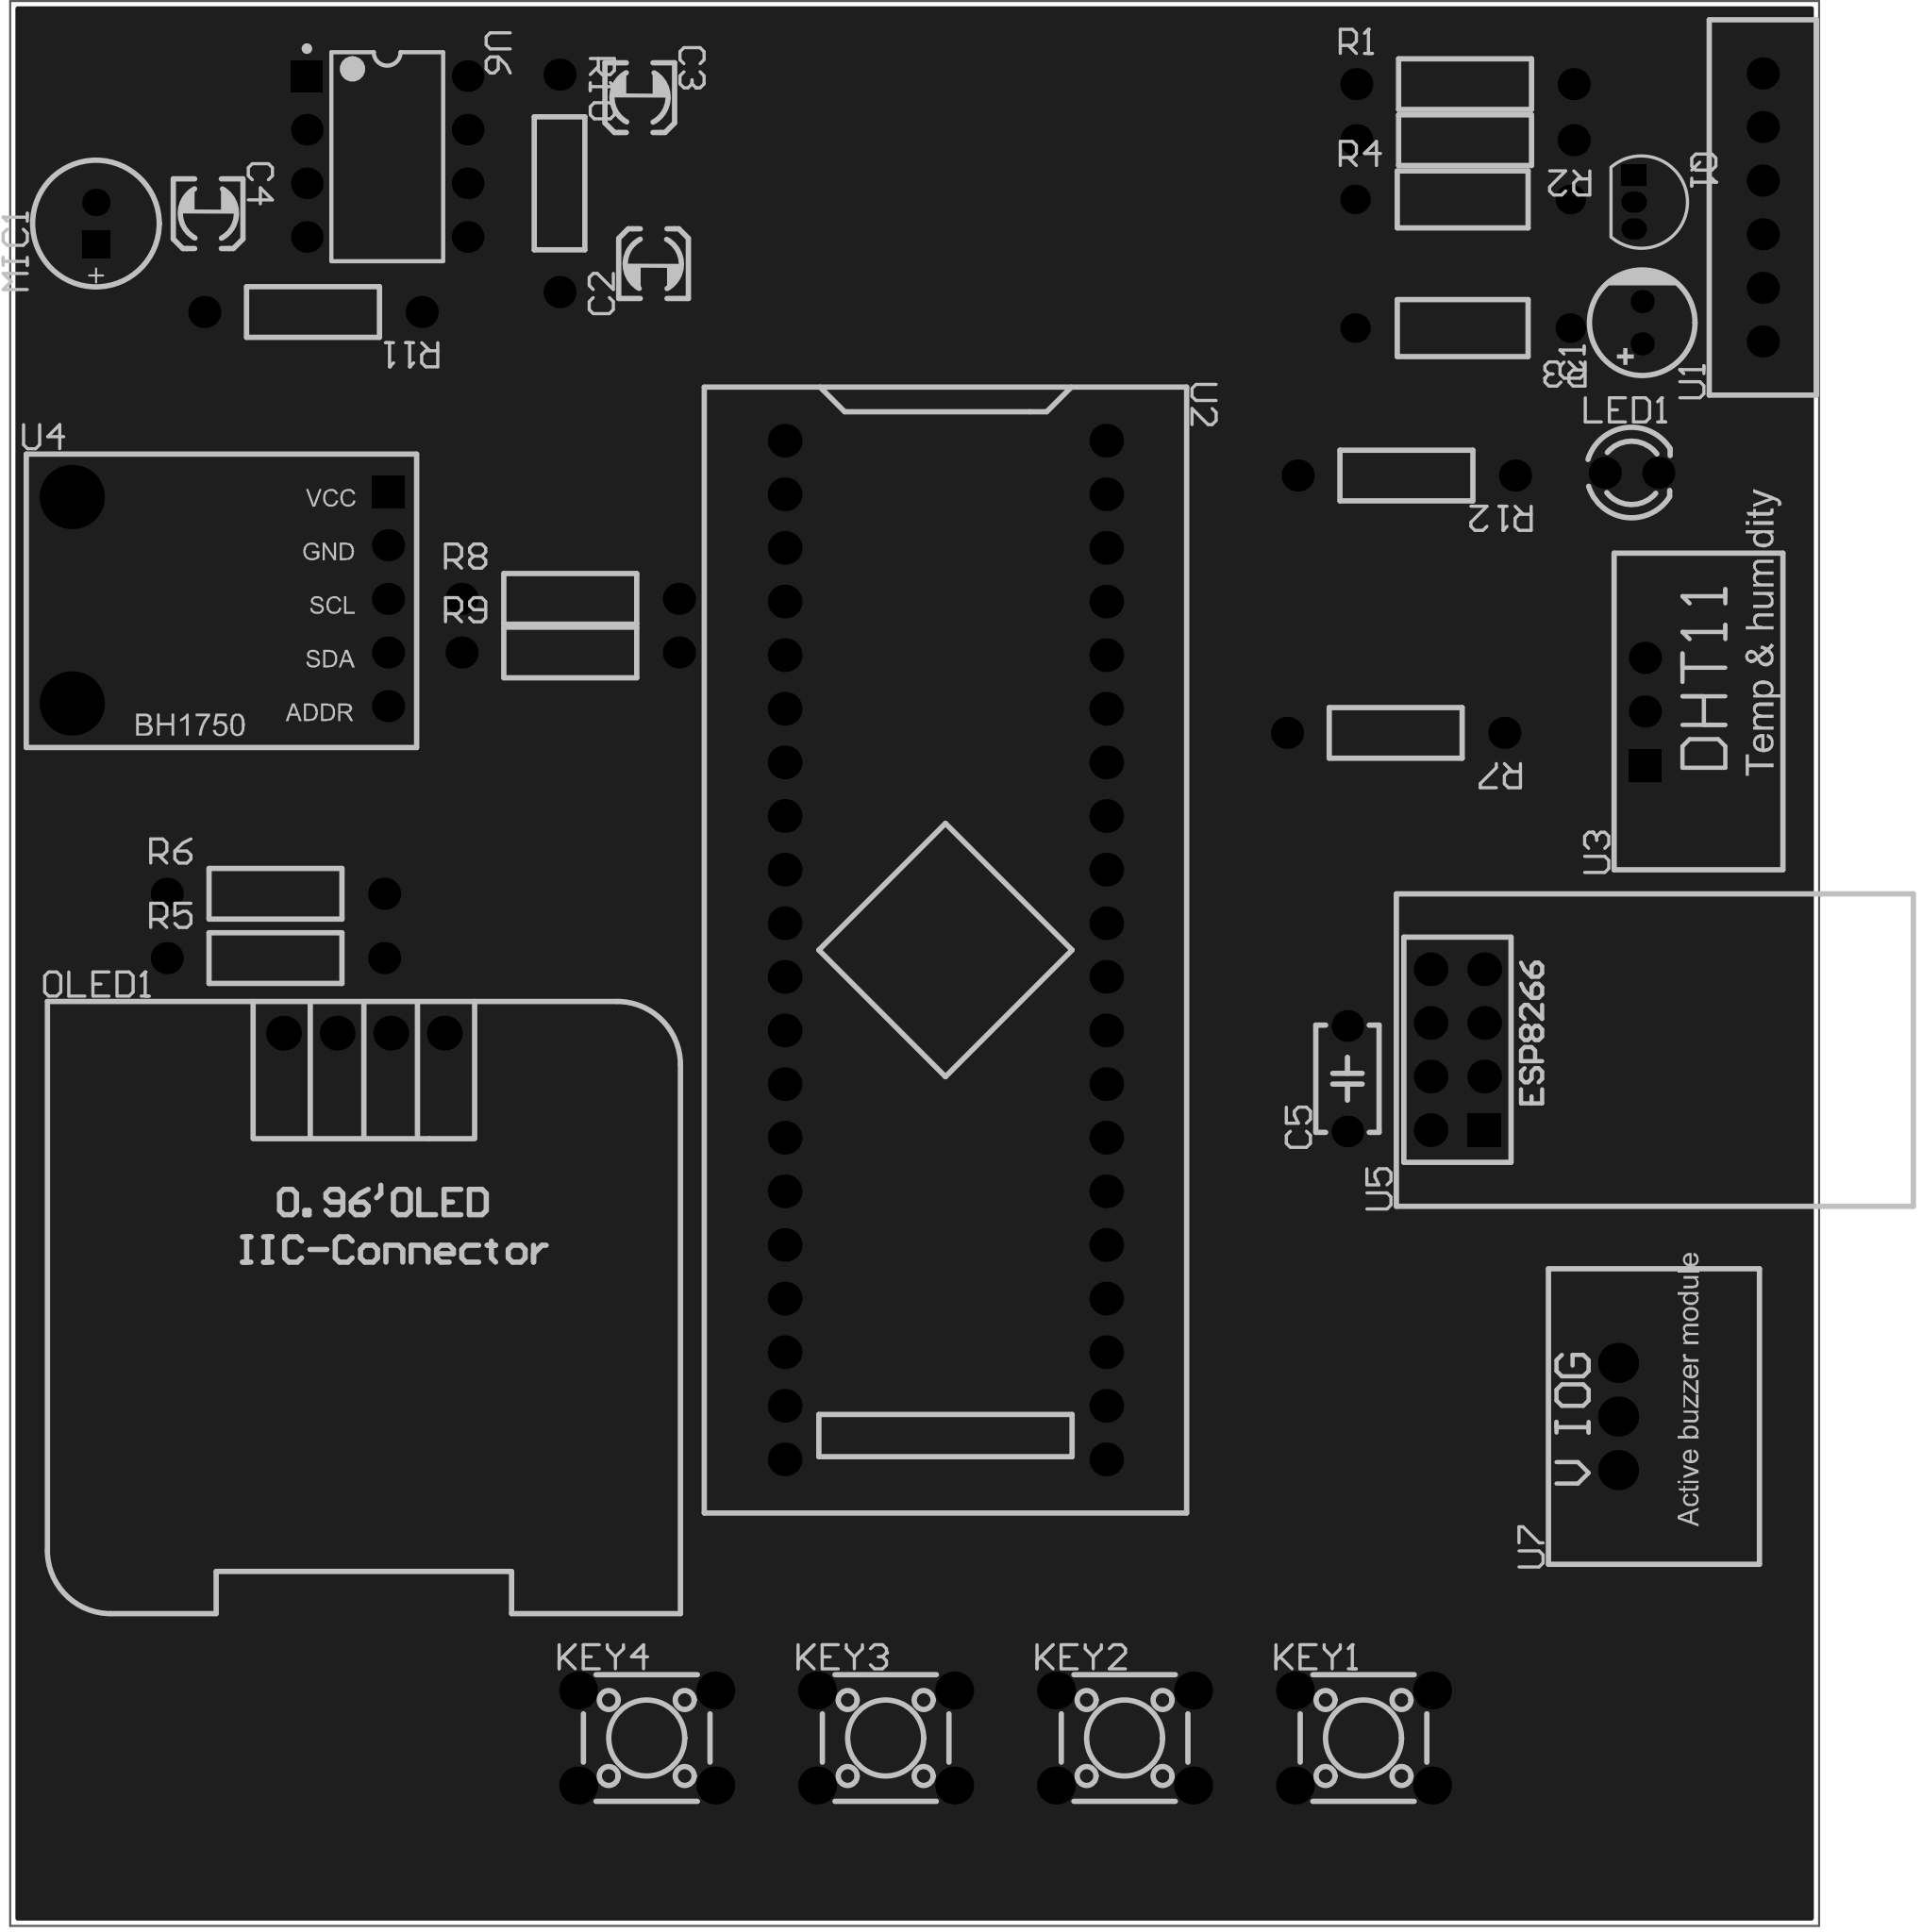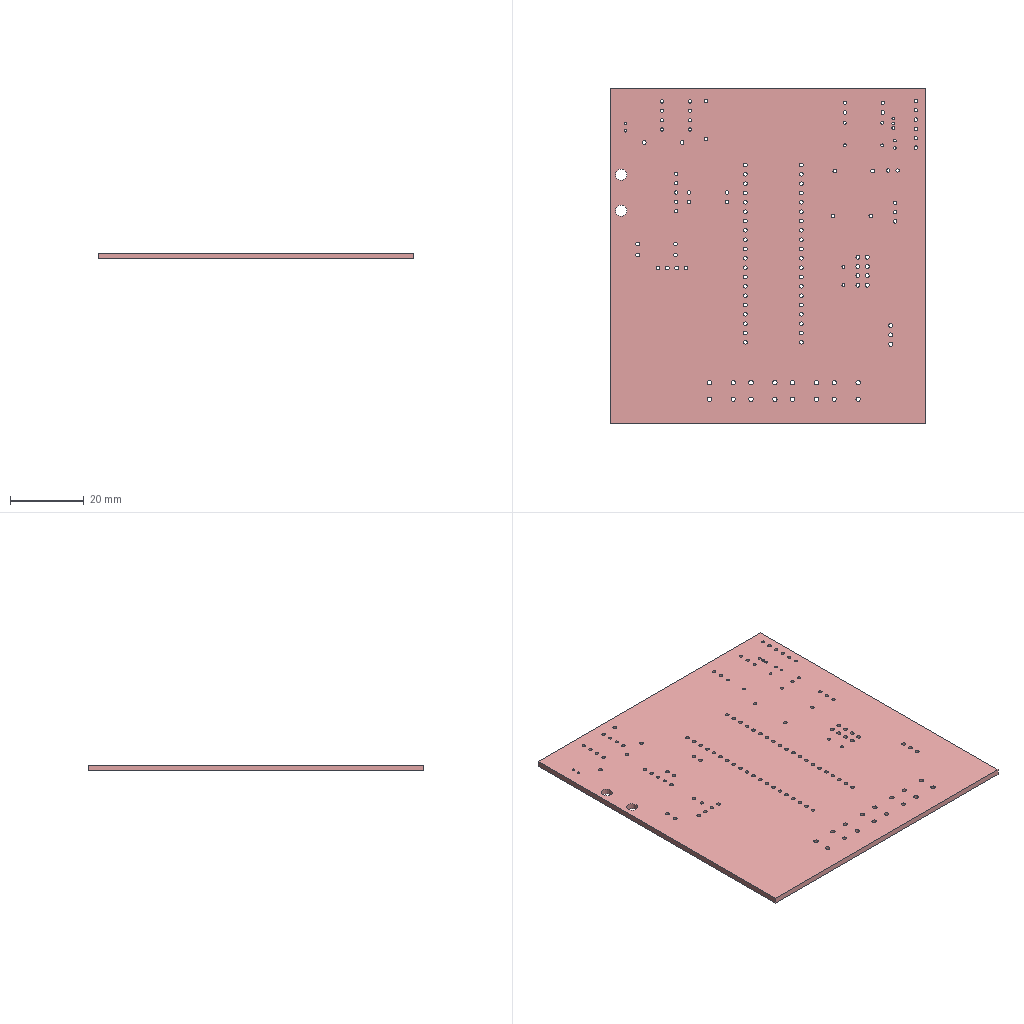Circuit board layout | Altium Designer | box 85.7 x 91.2 x 1.6 mm
Layer stack:
# Altium Designer layer stack of  (unit mm; dielectric type: 0 none, 1 core, 2 prepreg, 3 surface material)
index,name,kind,layer,copper_thickness_mm,dielectric_type,dielectric_thickness_mm,dielectric_material,dielectric_constant
0,Top Paste Mask Layer,other,,,,,,
1,Top Silkscreen Layer,other,,,,,,
2,Top Solder Mask Layer,dielectric,,,3,0.01,,3.3
3,Top Layer,copper,Top Layer,0.035,,,,
4,Dielectric1,dielectric,,,3,1.51,FR4,4.5
5,Bottom Layer,copper,Bottom Layer,0.035,,,,
6,Bottom Solder Mask Layer,dielectric,,,3,0.01,,3.3
7,Bottom Silkscreen Layer,other,,,,,,
8,Bottom Paste Mask Layer,other,,,,,,
# drill layer pairs: low layer,high layer
drill_pair,Top Layer,Bottom Layer
Part placement:
Designator,Comment,Layer,Footprint,Center-X(mm),Center-Y(mm),Rotation
C1,10uF,TopLayer,CAP-TH_BD5.0-P2.00-D0.5-FD,158.877,160.782,90
C2,10uF,TopLayer,C_Ele_SMD_3x5.4mm,112.028,163.581,90
C3,10uF,TopLayer,C_Ele_SMD_3x5.4mm,111.365,171.445,270
C4,10uF,TopLayer,C_Ele_SMD_3x5.4mm,90.909,165.947,270
C5,5pF,TopLayer,CAP-TH_L5.0-W3.0-P5.00-D0.6,144.907,124.968,90
KEY1,,TopLayer,SW-TH_4P-L6.0-W6.0-P4.50-LS6.5,145.669,93.736,0
KEY2,,TopLayer,SW-TH_4P-L6.0-W6.0-P4.50-LS6.5,134.346,93.736,0
KEY3,,TopLayer,SW-TH_4P-L6.0-W6.0-P4.50-LS6.5,123.023,93.736,0
KEY4,,TopLayer,SW-TH_4P-L6.0-W6.0-P4.50-LS6.5,111.7,93.736,0
LED1,,TopLayer,LED_TH-3mm,158.369,153.67,0
MIC1,MIC,TopLayer,MIC-TH_BD6.0-P2.00,85.598,165.481,90
OLED1,0.96OLED_4P_MODULE_JX,TopLayer,0.96OLED_4P,98.298,127.127,0
Q1,S8050,TopLayer,TO-92-3_L4.5-W3.5-P1.27-L,158.496,166.497,270
R1,10kΩ,TopLayer,Res_1/4W,150.48,172.085,0
R2,10kΩ,TopLayer,Res_1/4W,150.48,169.429,180
R3,10kΩ,TopLayer,RES-TH_BD2.7-L6.2-P10.20-D0.4,150.368,160.528,180
R4,1kΩ,TopLayer,RES-TH_BD2.7-L6.2-P10.20-D0.4,150.368,166.624,0
R5,10kΩ,TopLayer,Res_1/4W,94.107,130.683,0
R6,10kΩ,TopLayer,Res_1/4W,94.107,133.731,0
R7,4.7K,TopLayer,Res_1/4W,147.193,141.351,180
R8,10kΩ,TopLayer,Res_1/4W,108.077,147.701,0
R9,10kΩ,TopLayer,Res_1/4W,108.077,145.161,0
R10,3kΩ,TopLayer,Res_1/4W,107.569,167.386,270
R11,100kΩ,TopLayer,Res_1/4W,95.885,161.29,180
R12,10kΩ,TopLayer,Res_1/4W,147.701,153.543,180
U1,PM2.5 sensor_GP2Y1014AU,TopLayer,PM2.5传感器_GP2Y1014AU,164.592,166.243,90
U2,STM32F103C8T6-Card,TopLayer,CONN-TH_L53.3-W22.9_STM32F103C8T6-CARD,125.857,131.064,270
U3,DHT11,TopLayer,DHT11,159.004,142.367,90
U4,,TopLayer,BH1750光照传感器,91.948,147.701,0
U5,,TopLayer,ESP8266-1,150.119,126.342,90
U6,LM386N-3/NOPB,TopLayer,DIP-8_L9.8-W6.6-P2.54-LS7.6-BL,99.404,168.656,270
U7,,TopLayer,有源蜂鸣器模块,157.734,108.966,90
Pad and via stacks:
# Altium Designer via and pad stacks of  (unit mm). Each distinct definition once, with the count of objects using it.
# via: kind,start_layer,end_layer,hole_mm,diameter_mm,mode(0 simple;1 top-mid-bottom;2 full stack),diameter_per_layer,count,example_net
# pad: kind,layer,hole_mm,hole_type(0 round;1 square;2 slot),plating,top_size,top_shape(1 round;2 rect;3 octagon;9 rounded rect),mid_size,bottom_size,mode,footprint,size_per_layer,count,example
pad,Multi-Layer,0.7,0,plated,1.1x1.1,1,1.1x1.1,1.1x1.1,0,CAP-TH_BD5.0-P2.00-D0.5-FD,,2,C1.1
pad,Multi-Layer,0.8,0,plated,1.5x1.5,1,1.5x1.5,1.5x1.5,0,CAP-TH_L5.0-W3.0-P5.00-D0.6,,2,C5.2
pad,Multi-Layer,1.2,0,plated,1.8x1.8,1,1.8x1.8,1.8x1.8,0,SW-TH_4P-L6.0-W6.0-P4.50-LS6.5,,16,KEY1.1
pad,Multi-Layer,0.9144,0,plated,1.524x1.524,1,1.524x1.524,1.524x1.524,0,LED_TH-3mm,,2,LED1.1
pad,Multi-Layer,0.7,0,plated,1.3x1.3,2,1.3x1.3,1.3x1.3,0,MIC-TH_BD6.0-P2.00,,1,MIC1.1
pad,Multi-Layer,0.7,0,plated,1.3x1.3,1,1.3x1.3,1.3x1.3,0,MIC-TH_BD6.0-P2.00,,1,MIC1.2
pad,Multi-Layer,1,0,plated,1.65x1.65,1,1.65x1.65,1.65x1.65,0,0.96OLED_4P,,4,OLED1.4
pad,Multi-Layer,0.7,2,plated,1x1.2,2,1x1.2,1x1.2,0,TO-92-3_L4.5-W3.5-P1.27-L,,1,Q1.1
pad,Multi-Layer,0.7,2,plated,1x1.2,1,1x1.2,1x1.2,0,TO-92-3_L4.5-W3.5-P1.27-L,,2,Q1.2
pad,Multi-Layer,1,0,plated,1.524x1.524,1,1.524x1.524,1.524x1.524,0,Res_1/4W,,20,R1.1
pad,Multi-Layer,0.8,0,plated,1.4x1.4,1,1.4x1.4,1.4x1.4,0,RES-TH_BD2.7-L6.2-P10.20-D0.4,,4,R3.1
pad,Multi-Layer,0.9144,0,plated,1.524x1.524,1,1.524x1.524,1.524x1.524,0,PM2.5\u00B4\u00AB\u00B8\u00D0\u00C6\u00F7_GP2Y1014AU,,6,U1.1
pad,Multi-Layer,1,0,plated,1.6x1.6,1,1.6x1.6,1.6x1.6,0,CONN-TH_L53.3-W22.9_STM32F103C8T6-CARD,,40,U2.1
pad,Multi-Layer,0.9144,0,plated,1.524x1.524,1,1.524x1.524,1.524x1.524,0,DHT11,,2,U3.3
pad,Multi-Layer,0.9144,0,plated,1.524x1.524,2,1.524x1.524,1.524x1.524,0,DHT11,,1,U3.1
pad,Multi-Layer,3.048,0,unplated,3.048x3.048,1,3.048x3.048,3.048x3.048,0,BH1750\u00B9\u00E2\u00D5\u00D5\u00B4\u00AB\u00B8\u00D0\u00C6\u00F7,,2,U4.
pad,Multi-Layer,0.9144,0,plated,1.524x1.524,2,1.524x1.524,1.524x1.524,0,BH1750\u00B9\u00E2\u00D5\u00D5\u00B4\u00AB\u00B8\u00D0\u00C6\u00F7,,1,U4.1
pad,Multi-Layer,0.9144,0,plated,1.524x1.524,1,1.524x1.524,1.524x1.524,0,BH1750\u00B9\u00E2\u00D5\u00D5\u00B4\u00AB\u00B8\u00D0\u00C6\u00F7,,4,U4.4
pad,Multi-Layer,1.1,0,plated,1.6x1.6,2,1.6x1.6,1.6x1.6,0,ESP8266-1,,1,U5.1
pad,Multi-Layer,1.1,0,plated,1.6x1.6,1,1.6x1.6,1.6x1.6,0,ESP8266-1,,7,U5.2
pad,Multi-Layer,0.9,0,plated,1.5x1.5,2,1.5x1.5,1.5x1.5,0,DIP-8_L9.8-W6.6-P2.54-LS7.6-BL,,1,U6.1
pad,Multi-Layer,0.9,0,plated,1.5x1.5,1,1.5x1.5,1.5x1.5,0,DIP-8_L9.8-W6.6-P2.54-LS7.6-BL,,7,U6.2
pad,Multi-Layer,1.1,0,plated,1.9x1.9,1,1.9x1.9,1.9x1.9,0,\u00D3\u00D0\u00D4\u00B4\u00B7\u00E4\u00C3\u00F9\u00C6\u00F7\u00C4\u00A3\u00BF\u00E9,,3,U7.1
pad,Top Layer,0,0,plated,1.999x0.8001,2,1.999x0.8001,1.999x0.8001,0,C_Ele_SMD_3x5.4mm,,6,C2.1
Copper pours:
name,layer,net,type(0 solid;1 hatched;2 none)
Top Layer-GND,Top Layer,GND,0
Bottom Layer-GND,Bottom Layer,GND,0